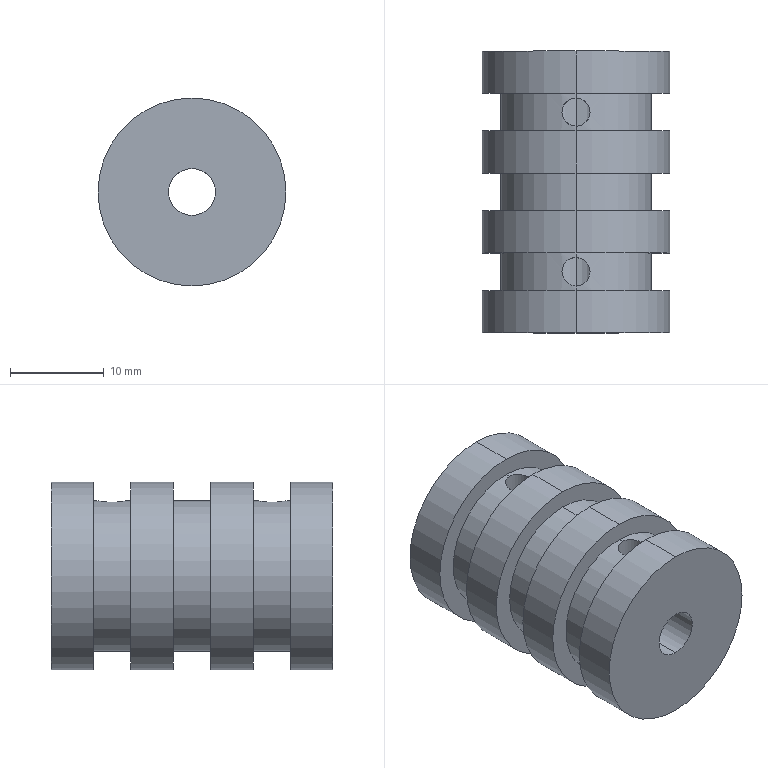Part | SolidWorks | features ICE 1, Revolution 1 | 1 solid | 31 faces | box 20 x 30 x 20 mm | volume 6534 mm3 | cylinder 22 | plane 9 | commonest cylinder face diameters 20 x8 16 x6 3 x4 5 x2 10 x2
STEP:
#1=CARTESIAN_POINT('',(0.,5.,8.));
#2=VERTEX_POINT('',#1);
#3=CARTESIAN_POINT('',(1.5,6.5,7.858));
#4=VERTEX_POINT('',#3);
#5=CARTESIAN_POINT('',(0.,5.,8.));
#6=CARTESIAN_POINT('',(0.09806,5.,8.));
#7=CARTESIAN_POINT('',(0.1977,5.01,7.998));
#8=CARTESIAN_POINT('',(0.3902,5.048,7.991));
#9=CARTESIAN_POINT('',(0.4838,5.077,7.986));
#10=CARTESIAN_POINT('',(0.7565,5.19,7.966));
#11=CARTESIAN_POINT('',(0.9215,5.3,7.948));
#12=CARTESIAN_POINT('',(1.131,5.509,7.92));
#13=CARTESIAN_POINT('',(1.193,5.585,7.911));
#14=CARTESIAN_POINT('',(1.301,5.747,7.894));
#15=CARTESIAN_POINT('',(1.348,5.835,7.886));
#16=CARTESIAN_POINT('',(1.423,6.016,7.872));
#17=CARTESIAN_POINT('',(1.452,6.11,7.867));
#18=CARTESIAN_POINT('',(1.49,6.302,7.86));
#19=CARTESIAN_POINT('',(1.5,6.402,7.858));
#20=CARTESIAN_POINT('',(1.5,6.5,7.858));
#21=B_SPLINE_CURVE_WITH_KNOTS('',3,(#5,#6,#7,#8,#9,#10,#11,#12,#13,#14,#15,#16,#17,#18,#19,#20),.UNSPECIFIED.,.F.,.F.,(4,2,2,2,2,2,2,4),(0.002351,0.002644,0.002938,0.003525,0.003819,0.004113,0.004406,0.0047),.UNSPECIFIED.);
#22=EDGE_CURVE('',#2,#4,#21,.T.);
#23=ORIENTED_EDGE('',*,*,#22,.T.);
#24=CARTESIAN_POINT('',(1.5,6.5,2.));
#25=VERTEX_POINT('',#24);
#26=CARTESIAN_POINT('',(1.5,6.5,10.001));
#27=DIRECTION('',(0.,0.,-1.));
#28=VECTOR('',#27,1000.);
#29=LINE('',#26,#28);
#30=EDGE_CURVE('',#4,#25,#29,.T.);
#31=ORIENTED_EDGE('',*,*,#30,.T.);
#32=CARTESIAN_POINT('',(0.,5.,2.5));
#33=VERTEX_POINT('',#32);
#34=CARTESIAN_POINT('',(1.5,6.5,2.));
#35=CARTESIAN_POINT('',(1.5,6.398,2.));
#36=CARTESIAN_POINT('',(1.49,6.298,2.008));
#37=CARTESIAN_POINT('',(1.45,6.103,2.037));
#38=CARTESIAN_POINT('',(1.42,6.007,2.058));
#39=CARTESIAN_POINT('',(1.306,5.737,2.134));
#40=CARTESIAN_POINT('',(1.197,5.576,2.2));
#41=CARTESIAN_POINT('',(0.994,5.373,2.295));
#42=CARTESIAN_POINT('',(0.9189,5.311,2.327));
#43=CARTESIAN_POINT('',(0.7595,5.203,2.383));
#44=CARTESIAN_POINT('',(0.6745,5.157,2.409));
#45=CARTESIAN_POINT('',(0.4928,5.08,2.453));
#46=CARTESIAN_POINT('',(0.3966,5.05,2.47));
#47=CARTESIAN_POINT('',(0.2019,5.01,2.494));
#48=CARTESIAN_POINT('',(0.1018,5.,2.5));
#49=CARTESIAN_POINT('',(0.,5.,2.5));
#50=B_SPLINE_CURVE_WITH_KNOTS('',3,(#34,#35,#36,#37,#38,#39,#40,#41,#42,#43,#44,#45,#46,#47,#48,#49),.UNSPECIFIED.,.F.,.F.,(4,2,2,2,2,2,2,4),(0.00481,0.005111,0.005411,0.006011,0.006311,0.006612,0.006912,0.007212),.UNSPECIFIED.);
#51=EDGE_CURVE('',#25,#33,#50,.T.);
#52=ORIENTED_EDGE('',*,*,#51,.T.);
#53=CARTESIAN_POINT('',(-1.5,6.5,2.));
#54=VERTEX_POINT('',#53);
#55=CARTESIAN_POINT('',(0.,5.,2.5));
#56=CARTESIAN_POINT('',(-0.1017,5.,2.5));
#57=CARTESIAN_POINT('',(-0.2015,5.01,2.494));
#58=CARTESIAN_POINT('',(-0.3974,5.05,2.47));
#59=CARTESIAN_POINT('',(-0.494,5.08,2.452));
#60=CARTESIAN_POINT('',(-0.7657,5.195,2.387));
#61=CARTESIAN_POINT('',(-0.9285,5.306,2.326));
#62=CARTESIAN_POINT('',(-1.131,5.51,2.231));
#63=CARTESIAN_POINT('',(-1.192,5.585,2.198));
#64=CARTESIAN_POINT('',(-1.299,5.744,2.137));
#65=CARTESIAN_POINT('',(-1.345,5.828,2.108));
#66=CARTESIAN_POINT('',(-1.421,6.008,2.058));
#67=CARTESIAN_POINT('',(-1.45,6.104,2.037));
#68=CARTESIAN_POINT('',(-1.49,6.298,2.008));
#69=CARTESIAN_POINT('',(-1.5,6.398,2.));
#70=CARTESIAN_POINT('',(-1.5,6.5,2.));
#71=B_SPLINE_CURVE_WITH_KNOTS('',3,(#55,#56,#57,#58,#59,#60,#61,#62,#63,#64,#65,#66,#67,#68,#69,#70),.UNSPECIFIED.,.F.,.F.,(4,2,2,2,2,2,2,4),(0.007212,0.007512,0.007812,0.008412,0.008712,0.009012,0.009312,0.009612),.UNSPECIFIED.);
#72=EDGE_CURVE('',#33,#54,#71,.T.);
#73=ORIENTED_EDGE('',*,*,#72,.T.);
#74=CARTESIAN_POINT('',(-1.5,6.5,7.858));
#75=VERTEX_POINT('',#74);
#76=CARTESIAN_POINT('',(-1.5,6.5,10.001));
#77=DIRECTION('',(0.,0.,-1.));
#78=VECTOR('',#77,1000.);
#79=LINE('',#76,#78);
#80=EDGE_CURVE('',#75,#54,#79,.T.);
#81=ORIENTED_EDGE('',*,*,#80,.F.);
#82=CARTESIAN_POINT('',(-1.5,6.5,7.858));
#83=CARTESIAN_POINT('',(-1.5,6.401,7.858));
#84=CARTESIAN_POINT('',(-1.49,6.303,7.86));
#85=CARTESIAN_POINT('',(-1.452,6.111,7.867));
#86=CARTESIAN_POINT('',(-1.423,6.015,7.873));
#87=CARTESIAN_POINT('',(-1.348,5.834,7.886));
#88=CARTESIAN_POINT('',(-1.301,5.748,7.894));
#89=CARTESIAN_POINT('',(-1.193,5.585,7.911));
#90=CARTESIAN_POINT('',(-1.129,5.508,7.92));
#91=CARTESIAN_POINT('',(-0.9221,5.301,7.948));
#92=CARTESIAN_POINT('',(-0.755,5.189,7.966));
#93=CARTESIAN_POINT('',(-0.394,5.04,7.992));
#94=CARTESIAN_POINT('',(-0.1962,5.,8.));
#95=CARTESIAN_POINT('',(0.,5.,8.));
#96=B_SPLINE_CURVE_WITH_KNOTS('',3,(#82,#83,#84,#85,#86,#87,#88,#89,#90,#91,#92,#93,#94,#95),.UNSPECIFIED.,.F.,.F.,(4,2,2,2,2,2,4),(0.,0.0002938,0.0005877,0.0008815,0.001175,0.001763,0.002351),.UNSPECIFIED.);
#97=EDGE_CURVE('',#75,#2,#96,.T.);
#98=ORIENTED_EDGE('',*,*,#97,.T.);
#99=EDGE_LOOP('',(#23,#31,#52,#73,#81,#98));
#100=FACE_OUTER_BOUND('',#99,.T.);
#101=CARTESIAN_POINT('',(0.,6.5,10.001));
#102=DIRECTION('',(0.,0.,-1.));
#103=DIRECTION('',(-1.,0.,0.));
#104=AXIS2_PLACEMENT_3D('',#101,#102,#103);
#105=CYLINDRICAL_SURFACE('',#104,1.5);
#106=ADVANCED_FACE('',(#100),#105,.F.);
#107=CARTESIAN_POINT('',(0.,22.,8.));
#108=VERTEX_POINT('',#107);
#109=CARTESIAN_POINT('',(1.5,23.5,7.858));
#110=VERTEX_POINT('',#109);
#111=CARTESIAN_POINT('',(0.,22.,8.));
#112=CARTESIAN_POINT('',(0.09806,22.,8.));
#113=CARTESIAN_POINT('',(0.1977,22.01,7.998));
#114=CARTESIAN_POINT('',(0.3902,22.048,7.991));
#115=CARTESIAN_POINT('',(0.4838,22.077,7.986));
#116=CARTESIAN_POINT('',(0.7565,22.19,7.966));
#117=CARTESIAN_POINT('',(0.9215,22.3,7.948));
#118=CARTESIAN_POINT('',(1.131,22.509,7.92));
#119=CARTESIAN_POINT('',(1.193,22.585,7.911));
#120=CARTESIAN_POINT('',(1.301,22.747,7.894));
#121=CARTESIAN_POINT('',(1.348,22.835,7.886));
#122=CARTESIAN_POINT('',(1.423,23.016,7.872));
#123=CARTESIAN_POINT('',(1.452,23.11,7.867));
#124=CARTESIAN_POINT('',(1.49,23.302,7.86));
#125=CARTESIAN_POINT('',(1.5,23.402,7.858));
#126=CARTESIAN_POINT('',(1.5,23.5,7.858));
#127=B_SPLINE_CURVE_WITH_KNOTS('',3,(#111,#112,#113,#114,#115,#116,#117,#118,#119,#120,#121,#122,#123,#124,#125,#126),.UNSPECIFIED.,.F.,.F.,(4,2,2,2,2,2,2,4),(0.002351,0.002644,0.002938,0.003525,0.003819,0.004113,0.004406,0.0047),.UNSPECIFIED.);
#128=EDGE_CURVE('',#108,#110,#127,.T.);
#129=ORIENTED_EDGE('',*,*,#128,.T.);
#130=CARTESIAN_POINT('',(1.5,23.5,4.77));
#131=VERTEX_POINT('',#130);
#132=CARTESIAN_POINT('',(1.5,23.5,10.001));
#133=DIRECTION('',(0.,0.,-1.));
#134=VECTOR('',#133,1000.);
#135=LINE('',#132,#134);
#136=EDGE_CURVE('',#110,#131,#135,.T.);
#137=ORIENTED_EDGE('',*,*,#136,.T.);
#138=CARTESIAN_POINT('',(0.,22.,5.));
#139=VERTEX_POINT('',#138);
#140=CARTESIAN_POINT('',(1.5,23.5,4.77));
#141=CARTESIAN_POINT('',(1.5,23.304,4.77));
#142=CARTESIAN_POINT('',(1.46,23.105,4.783));
#143=CARTESIAN_POINT('',(1.348,22.834,4.815));
#144=CARTESIAN_POINT('',(1.301,22.746,4.828));
#145=CARTESIAN_POINT('',(1.192,22.584,4.856));
#146=CARTESIAN_POINT('',(1.13,22.509,4.871));
#147=CARTESIAN_POINT('',(0.9225,22.301,4.916));
#148=CARTESIAN_POINT('',(0.759,22.191,4.945));
#149=CARTESIAN_POINT('',(0.4847,22.077,4.977));
#150=CARTESIAN_POINT('',(0.3908,22.048,4.986));
#151=CARTESIAN_POINT('',(0.1985,22.01,4.997));
#152=CARTESIAN_POINT('',(0.09886,22.,5.));
#153=CARTESIAN_POINT('',(0.,22.,5.));
#154=B_SPLINE_CURVE_WITH_KNOTS('',3,(#140,#141,#142,#143,#144,#145,#146,#147,#148,#149,#150,#151,#152,#153),.UNSPECIFIED.,.F.,.F.,(4,2,2,2,2,2,4),(0.004717,0.005306,0.005601,0.005896,0.006485,0.00678,0.007075),.UNSPECIFIED.);
#155=EDGE_CURVE('',#131,#139,#154,.T.);
#156=ORIENTED_EDGE('',*,*,#155,.T.);
#157=CARTESIAN_POINT('',(-1.5,23.5,4.77));
#158=VERTEX_POINT('',#157);
#159=CARTESIAN_POINT('',(0.,22.,5.));
#160=CARTESIAN_POINT('',(-0.09885,22.,5.));
#161=CARTESIAN_POINT('',(-0.1966,22.01,4.997));
#162=CARTESIAN_POINT('',(-0.3899,22.048,4.986));
#163=CARTESIAN_POINT('',(-0.4856,22.077,4.977));
#164=CARTESIAN_POINT('',(-0.7566,22.19,4.946));
#165=CARTESIAN_POINT('',(-0.9229,22.302,4.916));
#166=CARTESIAN_POINT('',(-1.129,22.508,4.871));
#167=CARTESIAN_POINT('',(-1.192,22.584,4.856));
#168=CARTESIAN_POINT('',(-1.301,22.747,4.828));
#169=CARTESIAN_POINT('',(-1.347,22.833,4.815));
#170=CARTESIAN_POINT('',(-1.422,23.014,4.794));
#171=CARTESIAN_POINT('',(-1.452,23.109,4.785));
#172=CARTESIAN_POINT('',(-1.49,23.302,4.773));
#173=CARTESIAN_POINT('',(-1.5,23.4,4.77));
#174=CARTESIAN_POINT('',(-1.5,23.5,4.77));
#175=B_SPLINE_CURVE_WITH_KNOTS('',3,(#159,#160,#161,#162,#163,#164,#165,#166,#167,#168,#169,#170,#171,#172,#173,#174),.UNSPECIFIED.,.F.,.F.,(4,2,2,2,2,2,2,4),(0.007075,0.00737,0.007664,0.008254,0.008548,0.008843,0.009138,0.009433),.UNSPECIFIED.);
#176=EDGE_CURVE('',#139,#158,#175,.T.);
#177=ORIENTED_EDGE('',*,*,#176,.T.);
#178=CARTESIAN_POINT('',(-1.5,23.5,7.858));
#179=VERTEX_POINT('',#178);
#180=CARTESIAN_POINT('',(-1.5,23.5,10.001));
#181=DIRECTION('',(0.,0.,-1.));
#182=VECTOR('',#181,1000.);
#183=LINE('',#180,#182);
#184=EDGE_CURVE('',#179,#158,#183,.T.);
#185=ORIENTED_EDGE('',*,*,#184,.F.);
#186=CARTESIAN_POINT('',(-1.5,23.5,7.858));
#187=CARTESIAN_POINT('',(-1.5,23.401,7.858));
#188=CARTESIAN_POINT('',(-1.49,23.303,7.86));
#189=CARTESIAN_POINT('',(-1.452,23.111,7.867));
#190=CARTESIAN_POINT('',(-1.423,23.015,7.873));
#191=CARTESIAN_POINT('',(-1.348,22.834,7.886));
#192=CARTESIAN_POINT('',(-1.301,22.748,7.894));
#193=CARTESIAN_POINT('',(-1.193,22.585,7.911));
#194=CARTESIAN_POINT('',(-1.129,22.508,7.92));
#195=CARTESIAN_POINT('',(-0.9221,22.301,7.948));
#196=CARTESIAN_POINT('',(-0.755,22.189,7.966));
#197=CARTESIAN_POINT('',(-0.394,22.04,7.992));
#198=CARTESIAN_POINT('',(-0.1962,22.,8.));
#199=CARTESIAN_POINT('',(0.,22.,8.));
#200=B_SPLINE_CURVE_WITH_KNOTS('',3,(#186,#187,#188,#189,#190,#191,#192,#193,#194,#195,#196,#197,#198,#199),.UNSPECIFIED.,.F.,.F.,(4,2,2,2,2,2,4),(0.,0.0002938,0.0005877,0.0008815,0.001175,0.001763,0.002351),.UNSPECIFIED.);
#201=EDGE_CURVE('',#179,#108,#200,.T.);
#202=ORIENTED_EDGE('',*,*,#201,.T.);
#203=EDGE_LOOP('',(#129,#137,#156,#177,#185,#202));
#204=FACE_OUTER_BOUND('',#203,.T.);
#205=CARTESIAN_POINT('',(0.,23.5,10.001));
#206=DIRECTION('',(0.,0.,-1.));
#207=DIRECTION('',(-1.,0.,0.));
#208=AXIS2_PLACEMENT_3D('',#205,#206,#207);
#209=CYLINDRICAL_SURFACE('',#208,1.5);
#210=ADVANCED_FACE('',(#204),#209,.F.);
#211=CARTESIAN_POINT('',(0.,30.,-10.));
#212=VERTEX_POINT('',#211);
#213=CARTESIAN_POINT('',(0.,30.,10.));
#214=VERTEX_POINT('',#213);
#215=CARTESIAN_POINT('',(0.,30.,0.));
#216=DIRECTION('',(0.,-1.,0.));
#217=DIRECTION('',(0.,0.,-1.));
#218=AXIS2_PLACEMENT_3D('',#215,#216,#217);
#219=CIRCLE('',#218,10.);
#220=EDGE_CURVE('',#212,#214,#219,.T.);
#221=ORIENTED_EDGE('',*,*,#220,.T.);
#222=CARTESIAN_POINT('',(0.,25.5,10.));
#223=VERTEX_POINT('',#222);
#224=CARTESIAN_POINT('',(0.,0.,10.));
#225=DIRECTION('',(0.,-1.,0.));
#226=VECTOR('',#225,1000.);
#227=LINE('',#224,#226);
#228=EDGE_CURVE('',#214,#223,#227,.T.);
#229=ORIENTED_EDGE('',*,*,#228,.T.);
#230=CARTESIAN_POINT('',(0.,25.5,-10.));
#231=VERTEX_POINT('',#230);
#232=CARTESIAN_POINT('',(0.,25.5,0.));
#233=DIRECTION('',(0.,-1.,0.));
#234=DIRECTION('',(0.,0.,-1.));
#235=AXIS2_PLACEMENT_3D('',#232,#233,#234);
#236=CIRCLE('',#235,10.);
#237=EDGE_CURVE('',#231,#223,#236,.T.);
#238=ORIENTED_EDGE('',*,*,#237,.F.);
#239=CARTESIAN_POINT('',(0.,0.,-10.));
#240=DIRECTION('',(0.,-1.,0.));
#241=VECTOR('',#240,1000.);
#242=LINE('',#239,#241);
#243=EDGE_CURVE('',#212,#231,#242,.T.);
#244=ORIENTED_EDGE('',*,*,#243,.F.);
#245=EDGE_LOOP('',(#221,#229,#238,#244));
#246=FACE_OUTER_BOUND('',#245,.T.);
#247=CARTESIAN_POINT('',(0.,0.,0.));
#248=DIRECTION('',(0.,-1.,0.));
#249=DIRECTION('',(0.,0.,-1.));
#250=AXIS2_PLACEMENT_3D('',#247,#248,#249);
#251=CYLINDRICAL_SURFACE('',#250,10.);
#252=ADVANCED_FACE('',(#246),#251,.T.);
#253=CARTESIAN_POINT('',(0.,21.5,-10.));
#254=VERTEX_POINT('',#253);
#255=CARTESIAN_POINT('',(0.,21.5,10.));
#256=VERTEX_POINT('',#255);
#257=CARTESIAN_POINT('',(0.,21.5,0.));
#258=DIRECTION('',(0.,-1.,0.));
#259=DIRECTION('',(0.,0.,-1.));
#260=AXIS2_PLACEMENT_3D('',#257,#258,#259);
#261=CIRCLE('',#260,10.);
#262=EDGE_CURVE('',#254,#256,#261,.T.);
#263=ORIENTED_EDGE('',*,*,#262,.T.);
#264=CARTESIAN_POINT('',(0.,17.,10.));
#265=VERTEX_POINT('',#264);
#266=CARTESIAN_POINT('',(0.,0.,10.));
#267=DIRECTION('',(0.,-1.,0.));
#268=VECTOR('',#267,1000.);
#269=LINE('',#266,#268);
#270=EDGE_CURVE('',#256,#265,#269,.T.);
#271=ORIENTED_EDGE('',*,*,#270,.T.);
#272=CARTESIAN_POINT('',(0.,17.,-10.));
#273=VERTEX_POINT('',#272);
#274=CARTESIAN_POINT('',(0.,17.,0.));
#275=DIRECTION('',(0.,-1.,0.));
#276=DIRECTION('',(0.,0.,-1.));
#277=AXIS2_PLACEMENT_3D('',#274,#275,#276);
#278=CIRCLE('',#277,10.);
#279=EDGE_CURVE('',#273,#265,#278,.T.);
#280=ORIENTED_EDGE('',*,*,#279,.F.);
#281=CARTESIAN_POINT('',(0.,0.,-10.));
#282=DIRECTION('',(0.,-1.,0.));
#283=VECTOR('',#282,1000.);
#284=LINE('',#281,#283);
#285=EDGE_CURVE('',#254,#273,#284,.T.);
#286=ORIENTED_EDGE('',*,*,#285,.F.);
#287=EDGE_LOOP('',(#263,#271,#280,#286));
#288=FACE_OUTER_BOUND('',#287,.T.);
#289=CARTESIAN_POINT('',(0.,0.,0.));
#290=DIRECTION('',(0.,-1.,0.));
#291=DIRECTION('',(0.,0.,-1.));
#292=AXIS2_PLACEMENT_3D('',#289,#290,#291);
#293=CYLINDRICAL_SURFACE('',#292,10.);
#294=ADVANCED_FACE('',(#288),#293,.T.);
#295=CARTESIAN_POINT('',(0.,17.,-8.));
#296=VERTEX_POINT('',#295);
#297=CARTESIAN_POINT('',(0.,17.,8.));
#298=VERTEX_POINT('',#297);
#299=CARTESIAN_POINT('',(0.,17.,0.));
#300=DIRECTION('',(0.,-1.,0.));
#301=DIRECTION('',(0.,0.,-1.));
#302=AXIS2_PLACEMENT_3D('',#299,#300,#301);
#303=CIRCLE('',#302,8.);
#304=EDGE_CURVE('',#296,#298,#303,.T.);
#305=ORIENTED_EDGE('',*,*,#304,.T.);
#306=CARTESIAN_POINT('',(0.,13.,8.));
#307=VERTEX_POINT('',#306);
#308=CARTESIAN_POINT('',(0.,0.,8.));
#309=DIRECTION('',(0.,-1.,0.));
#310=VECTOR('',#309,1000.);
#311=LINE('',#308,#310);
#312=EDGE_CURVE('',#298,#307,#311,.T.);
#313=ORIENTED_EDGE('',*,*,#312,.T.);
#314=CARTESIAN_POINT('',(0.,13.,-8.));
#315=VERTEX_POINT('',#314);
#316=CARTESIAN_POINT('',(0.,13.,0.));
#317=DIRECTION('',(0.,-1.,0.));
#318=DIRECTION('',(0.,0.,-1.));
#319=AXIS2_PLACEMENT_3D('',#316,#317,#318);
#320=CIRCLE('',#319,8.);
#321=EDGE_CURVE('',#315,#307,#320,.T.);
#322=ORIENTED_EDGE('',*,*,#321,.F.);
#323=CARTESIAN_POINT('',(0.,0.,-8.));
#324=DIRECTION('',(0.,-1.,0.));
#325=VECTOR('',#324,1000.);
#326=LINE('',#323,#325);
#327=EDGE_CURVE('',#296,#315,#326,.T.);
#328=ORIENTED_EDGE('',*,*,#327,.F.);
#329=EDGE_LOOP('',(#305,#313,#322,#328));
#330=FACE_OUTER_BOUND('',#329,.T.);
#331=CARTESIAN_POINT('',(0.,0.,0.));
#332=DIRECTION('',(0.,-1.,0.));
#333=DIRECTION('',(0.,0.,-1.));
#334=AXIS2_PLACEMENT_3D('',#331,#332,#333);
#335=CYLINDRICAL_SURFACE('',#334,8.);
#336=ADVANCED_FACE('',(#330),#335,.T.);
#337=CARTESIAN_POINT('',(0.,13.,-10.));
#338=VERTEX_POINT('',#337);
#339=CARTESIAN_POINT('',(0.,13.,10.));
#340=VERTEX_POINT('',#339);
#341=CARTESIAN_POINT('',(0.,13.,0.));
#342=DIRECTION('',(0.,-1.,0.));
#343=DIRECTION('',(0.,0.,-1.));
#344=AXIS2_PLACEMENT_3D('',#341,#342,#343);
#345=CIRCLE('',#344,10.);
#346=EDGE_CURVE('',#338,#340,#345,.T.);
#347=ORIENTED_EDGE('',*,*,#346,.T.);
#348=CARTESIAN_POINT('',(0.,8.5,10.));
#349=VERTEX_POINT('',#348);
#350=CARTESIAN_POINT('',(0.,0.,10.));
#351=DIRECTION('',(0.,-1.,0.));
#352=VECTOR('',#351,1000.);
#353=LINE('',#350,#352);
#354=EDGE_CURVE('',#340,#349,#353,.T.);
#355=ORIENTED_EDGE('',*,*,#354,.T.);
#356=CARTESIAN_POINT('',(0.,8.5,-10.));
#357=VERTEX_POINT('',#356);
#358=CARTESIAN_POINT('',(0.,8.5,0.));
#359=DIRECTION('',(0.,-1.,0.));
#360=DIRECTION('',(0.,0.,-1.));
#361=AXIS2_PLACEMENT_3D('',#358,#359,#360);
#362=CIRCLE('',#361,10.);
#363=EDGE_CURVE('',#357,#349,#362,.T.);
#364=ORIENTED_EDGE('',*,*,#363,.F.);
#365=CARTESIAN_POINT('',(0.,0.,-10.));
#366=DIRECTION('',(0.,-1.,0.));
#367=VECTOR('',#366,1000.);
#368=LINE('',#365,#367);
#369=EDGE_CURVE('',#338,#357,#368,.T.);
#370=ORIENTED_EDGE('',*,*,#369,.F.);
#371=EDGE_LOOP('',(#347,#355,#364,#370));
#372=FACE_OUTER_BOUND('',#371,.T.);
#373=CARTESIAN_POINT('',(0.,0.,0.));
#374=DIRECTION('',(0.,-1.,0.));
#375=DIRECTION('',(0.,0.,-1.));
#376=AXIS2_PLACEMENT_3D('',#373,#374,#375);
#377=CYLINDRICAL_SURFACE('',#376,10.);
#378=ADVANCED_FACE('',(#372),#377,.T.);
#379=CARTESIAN_POINT('',(0.,4.5,-10.));
#380=VERTEX_POINT('',#379);
#381=CARTESIAN_POINT('',(0.,4.5,10.));
#382=VERTEX_POINT('',#381);
#383=CARTESIAN_POINT('',(0.,4.5,0.));
#384=DIRECTION('',(0.,-1.,0.));
#385=DIRECTION('',(0.,0.,-1.));
#386=AXIS2_PLACEMENT_3D('',#383,#384,#385);
#387=CIRCLE('',#386,10.);
#388=EDGE_CURVE('',#380,#382,#387,.T.);
#389=ORIENTED_EDGE('',*,*,#388,.T.);
#390=CARTESIAN_POINT('',(0.,0.,10.));
#391=VERTEX_POINT('',#390);
#392=CARTESIAN_POINT('',(0.,0.,10.));
#393=DIRECTION('',(0.,-1.,0.));
#394=VECTOR('',#393,1000.);
#395=LINE('',#392,#394);
#396=EDGE_CURVE('',#382,#391,#395,.T.);
#397=ORIENTED_EDGE('',*,*,#396,.T.);
#398=CARTESIAN_POINT('',(0.,0.,-10.));
#399=VERTEX_POINT('',#398);
#400=CARTESIAN_POINT('',(0.,0.,0.));
#401=DIRECTION('',(0.,-1.,0.));
#402=DIRECTION('',(0.,0.,-1.));
#403=AXIS2_PLACEMENT_3D('',#400,#401,#402);
#404=CIRCLE('',#403,10.);
#405=EDGE_CURVE('',#399,#391,#404,.T.);
#406=ORIENTED_EDGE('',*,*,#405,.F.);
#407=CARTESIAN_POINT('',(0.,0.,-10.));
#408=DIRECTION('',(0.,-1.,0.));
#409=VECTOR('',#408,1000.);
#410=LINE('',#407,#409);
#411=EDGE_CURVE('',#380,#399,#410,.T.);
#412=ORIENTED_EDGE('',*,*,#411,.F.);
#413=EDGE_LOOP('',(#389,#397,#406,#412));
#414=FACE_OUTER_BOUND('',#413,.T.);
#415=CARTESIAN_POINT('',(0.,0.,0.));
#416=DIRECTION('',(0.,-1.,0.));
#417=DIRECTION('',(0.,0.,-1.));
#418=AXIS2_PLACEMENT_3D('',#415,#416,#417);
#419=CYLINDRICAL_SURFACE('',#418,10.);
#420=ADVANCED_FACE('',(#414),#419,.T.);
#421=CARTESIAN_POINT('',(0.,30.,5.));
#422=VERTEX_POINT('',#421);
#423=CARTESIAN_POINT('',(0.,30.,-5.));
#424=VERTEX_POINT('',#423);
#425=CARTESIAN_POINT('',(0.,30.,0.));
#426=DIRECTION('',(0.,-1.,0.));
#427=DIRECTION('',(0.,0.,-1.));
#428=AXIS2_PLACEMENT_3D('',#425,#426,#427);
#429=CIRCLE('',#428,5.);
#430=EDGE_CURVE('',#422,#424,#429,.T.);
#431=ORIENTED_EDGE('',*,*,#430,.F.);
#432=CARTESIAN_POINT('',(0.,25.,5.));
#433=VERTEX_POINT('',#432);
#434=CARTESIAN_POINT('',(0.,0.,5.));
#435=DIRECTION('',(0.,-1.,0.));
#436=VECTOR('',#435,1000.);
#437=LINE('',#434,#436);
#438=EDGE_CURVE('',#422,#433,#437,.T.);
#439=ORIENTED_EDGE('',*,*,#438,.T.);
#440=CARTESIAN_POINT('',(-1.5,23.5,4.77));
#441=CARTESIAN_POINT('',(-1.5,23.6,4.77));
#442=CARTESIAN_POINT('',(-1.49,23.698,4.773));
#443=CARTESIAN_POINT('',(-1.452,23.89,4.785));
#444=CARTESIAN_POINT('',(-1.423,23.986,4.794));
#445=CARTESIAN_POINT('',(-1.347,24.167,4.815));
#446=CARTESIAN_POINT('',(-1.301,24.253,4.828));
#447=CARTESIAN_POINT('',(-1.192,24.416,4.856));
#448=CARTESIAN_POINT('',(-1.129,24.492,4.871));
#449=CARTESIAN_POINT('',(-0.9226,24.699,4.916));
#450=CARTESIAN_POINT('',(-0.7561,24.81,4.946));
#451=CARTESIAN_POINT('',(-0.3953,24.96,4.988));
#452=CARTESIAN_POINT('',(-0.197,25.,5.));
#453=CARTESIAN_POINT('',(0.,25.,5.));
#454=B_SPLINE_CURVE_WITH_KNOTS('',3,(#440,#441,#442,#443,#444,#445,#446,#447,#448,#449,#450,#451,#452,#453),.UNSPECIFIED.,.F.,.F.,(4,2,2,2,2,2,4),(0.,0.0002949,0.0005898,0.0008847,0.00118,0.001769,0.002359),.UNSPECIFIED.);
#455=EDGE_CURVE('',#158,#433,#454,.T.);
#456=ORIENTED_EDGE('',*,*,#455,.F.);
#457=ORIENTED_EDGE('',*,*,#176,.F.);
#458=CARTESIAN_POINT('',(0.,15.,5.));
#459=VERTEX_POINT('',#458);
#460=CARTESIAN_POINT('',(0.,0.,5.));
#461=DIRECTION('',(0.,-1.,0.));
#462=VECTOR('',#461,1000.);
#463=LINE('',#460,#462);
#464=EDGE_CURVE('',#139,#459,#463,.T.);
#465=ORIENTED_EDGE('',*,*,#464,.T.);
#466=CARTESIAN_POINT('',(0.,15.,-5.));
#467=VERTEX_POINT('',#466);
#468=CARTESIAN_POINT('',(0.,15.,0.));
#469=DIRECTION('',(0.,-1.,0.));
#470=DIRECTION('',(0.,0.,-1.));
#471=AXIS2_PLACEMENT_3D('',#468,#469,#470);
#472=CIRCLE('',#471,5.);
#473=EDGE_CURVE('',#459,#467,#472,.T.);
#474=ORIENTED_EDGE('',*,*,#473,.T.);
#475=CARTESIAN_POINT('',(0.,0.,-5.));
#476=DIRECTION('',(0.,-1.,0.));
#477=VECTOR('',#476,1000.);
#478=LINE('',#475,#477);
#479=EDGE_CURVE('',#424,#467,#478,.T.);
#480=ORIENTED_EDGE('',*,*,#479,.F.);
#481=EDGE_LOOP('',(#431,#439,#456,#457,#465,#474,#480));
#482=FACE_OUTER_BOUND('',#481,.T.);
#483=CARTESIAN_POINT('',(0.,0.,0.));
#484=DIRECTION('',(0.,-1.,0.));
#485=DIRECTION('',(0.,0.,-1.));
#486=AXIS2_PLACEMENT_3D('',#483,#484,#485);
#487=CYLINDRICAL_SURFACE('',#486,5.);
#488=ADVANCED_FACE('',(#482),#487,.F.);
#489=CARTESIAN_POINT('',(0.,25.5,-8.));
#490=VERTEX_POINT('',#489);
#491=CARTESIAN_POINT('',(0.,25.5,8.));
#492=VERTEX_POINT('',#491);
#493=CARTESIAN_POINT('',(0.,25.5,0.));
#494=DIRECTION('',(0.,-1.,0.));
#495=DIRECTION('',(0.,0.,-1.));
#496=AXIS2_PLACEMENT_3D('',#493,#494,#495);
#497=CIRCLE('',#496,8.);
#498=EDGE_CURVE('',#490,#492,#497,.T.);
#499=ORIENTED_EDGE('',*,*,#498,.T.);
#500=CARTESIAN_POINT('',(0.,25.,8.));
#501=VERTEX_POINT('',#500);
#502=CARTESIAN_POINT('',(0.,0.,8.));
#503=DIRECTION('',(0.,-1.,0.));
#504=VECTOR('',#503,1000.);
#505=LINE('',#502,#504);
#506=EDGE_CURVE('',#492,#501,#505,.T.);
#507=ORIENTED_EDGE('',*,*,#506,.T.);
#508=CARTESIAN_POINT('',(1.5,23.5,7.858));
#509=CARTESIAN_POINT('',(1.5,23.696,7.858));
#510=CARTESIAN_POINT('',(1.461,23.894,7.866));
#511=CARTESIAN_POINT('',(1.311,24.255,7.892));
#512=CARTESIAN_POINT('',(1.199,24.422,7.911));
#513=CARTESIAN_POINT('',(0.9919,24.629,7.939));
#514=CARTESIAN_POINT('',(0.9149,24.693,7.948));
#515=CARTESIAN_POINT('',(0.7523,24.801,7.965));
#516=CARTESIAN_POINT('',(0.6663,24.848,7.973));
#517=CARTESIAN_POINT('',(0.3933,24.961,7.992));
#518=CARTESIAN_POINT('',(0.1982,25.,8.));
#519=CARTESIAN_POINT('',(0.,25.,8.));
#520=B_SPLINE_CURVE_WITH_KNOTS('',3,(#508,#509,#510,#511,#512,#513,#514,#515,#516,#517,#518,#519),.UNSPECIFIED.,.F.,.F.,(4,2,2,2,2,4),(0.0047,0.005288,0.005875,0.006169,0.006463,0.00705),.UNSPECIFIED.);
#521=EDGE_CURVE('',#110,#501,#520,.T.);
#522=ORIENTED_EDGE('',*,*,#521,.F.);
#523=ORIENTED_EDGE('',*,*,#128,.F.);
#524=CARTESIAN_POINT('',(0.,21.5,8.));
#525=VERTEX_POINT('',#524);
#526=CARTESIAN_POINT('',(0.,0.,8.));
#527=DIRECTION('',(0.,-1.,0.));
#528=VECTOR('',#527,1000.);
#529=LINE('',#526,#528);
#530=EDGE_CURVE('',#108,#525,#529,.T.);
#531=ORIENTED_EDGE('',*,*,#530,.T.);
#532=CARTESIAN_POINT('',(0.,21.5,-8.));
#533=VERTEX_POINT('',#532);
#534=CARTESIAN_POINT('',(0.,21.5,0.));
#535=DIRECTION('',(0.,-1.,0.));
#536=DIRECTION('',(0.,0.,-1.));
#537=AXIS2_PLACEMENT_3D('',#534,#535,#536);
#538=CIRCLE('',#537,8.);
#539=EDGE_CURVE('',#533,#525,#538,.T.);
#540=ORIENTED_EDGE('',*,*,#539,.F.);
#541=CARTESIAN_POINT('',(0.,0.,-8.));
#542=DIRECTION('',(0.,-1.,0.));
#543=VECTOR('',#542,1000.);
#544=LINE('',#541,#543);
#545=EDGE_CURVE('',#490,#533,#544,.T.);
#546=ORIENTED_EDGE('',*,*,#545,.F.);
#547=EDGE_LOOP('',(#499,#507,#522,#523,#531,#540,#546));
#548=FACE_OUTER_BOUND('',#547,.T.);
#549=CARTESIAN_POINT('',(0.,0.,0.));
#550=DIRECTION('',(0.,-1.,0.));
#551=DIRECTION('',(0.,0.,-1.));
#552=AXIS2_PLACEMENT_3D('',#549,#550,#551);
#553=CYLINDRICAL_SURFACE('',#552,8.);
#554=ADVANCED_FACE('',(#548),#553,.T.);
#555=CARTESIAN_POINT('',(0.,15.,2.5));
#556=VERTEX_POINT('',#555);
#557=CARTESIAN_POINT('',(0.,15.,-2.5));
#558=VERTEX_POINT('',#557);
#559=CARTESIAN_POINT('',(0.,15.,0.));
#560=DIRECTION('',(0.,-1.,0.));
#561=DIRECTION('',(0.,0.,-1.));
#562=AXIS2_PLACEMENT_3D('',#559,#560,#561);
#563=CIRCLE('',#562,2.5);
#564=EDGE_CURVE('',#556,#558,#563,.T.);
#565=ORIENTED_EDGE('',*,*,#564,.F.);
#566=CARTESIAN_POINT('',(0.,8.,2.5));
#567=VERTEX_POINT('',#566);
#568=CARTESIAN_POINT('',(0.,0.,2.5));
#569=DIRECTION('',(0.,-1.,0.));
#570=VECTOR('',#569,1000.);
#571=LINE('',#568,#570);
#572=EDGE_CURVE('',#556,#567,#571,.T.);
#573=ORIENTED_EDGE('',*,*,#572,.T.);
#574=CARTESIAN_POINT('',(-1.5,6.5,2.));
#575=CARTESIAN_POINT('',(-1.5,6.602,2.));
#576=CARTESIAN_POINT('',(-1.49,6.702,2.008));
#577=CARTESIAN_POINT('',(-1.45,6.897,2.037));
#578=CARTESIAN_POINT('',(-1.42,6.993,2.058));
#579=CARTESIAN_POINT('',(-1.306,7.263,2.133));
#580=CARTESIAN_POINT('',(-1.197,7.424,2.2));
#581=CARTESIAN_POINT('',(-0.9943,7.627,2.295));
#582=CARTESIAN_POINT('',(-0.9191,7.689,2.326));
#583=CARTESIAN_POINT('',(-0.7589,7.797,2.384));
#584=CARTESIAN_POINT('',(-0.6739,7.844,2.409));
#585=CARTESIAN_POINT('',(-0.4932,7.92,2.453));
#586=CARTESIAN_POINT('',(-0.3963,7.95,2.47));
#587=CARTESIAN_POINT('',(-0.2008,7.99,2.494));
#588=CARTESIAN_POINT('',(-0.1013,8.,2.5));
#589=CARTESIAN_POINT('',(0.,8.,2.5));
#590=B_SPLINE_CURVE_WITH_KNOTS('',3,(#574,#575,#576,#577,#578,#579,#580,#581,#582,#583,#584,#585,#586,#587,#588,#589),.UNSPECIFIED.,.F.,.F.,(4,2,2,2,2,2,2,4),(0.,0.000301,0.000602,0.001204,0.001505,0.001806,0.002107,0.002408),.UNSPECIFIED.);
#591=EDGE_CURVE('',#54,#567,#590,.T.);
#592=ORIENTED_EDGE('',*,*,#591,.F.);
#593=ORIENTED_EDGE('',*,*,#72,.F.);
#594=CARTESIAN_POINT('',(0.,0.,2.5));
#595=VERTEX_POINT('',#594);
#596=CARTESIAN_POINT('',(0.,0.,2.5));
#597=DIRECTION('',(0.,-1.,0.));
#598=VECTOR('',#597,1000.);
#599=LINE('',#596,#598);
#600=EDGE_CURVE('',#33,#595,#599,.T.);
#601=ORIENTED_EDGE('',*,*,#600,.T.);
#602=CARTESIAN_POINT('',(0.,0.,-2.5));
#603=VERTEX_POINT('',#602);
#604=CARTESIAN_POINT('',(0.,0.,0.));
#605=DIRECTION('',(0.,-1.,0.));
#606=DIRECTION('',(0.,0.,-1.));
#607=AXIS2_PLACEMENT_3D('',#604,#605,#606);
#608=CIRCLE('',#607,2.5);
#609=EDGE_CURVE('',#595,#603,#608,.T.);
#610=ORIENTED_EDGE('',*,*,#609,.T.);
#611=CARTESIAN_POINT('',(0.,0.,-2.5));
#612=DIRECTION('',(0.,-1.,0.));
#613=VECTOR('',#612,1000.);
#614=LINE('',#611,#613);
#615=EDGE_CURVE('',#558,#603,#614,.T.);
#616=ORIENTED_EDGE('',*,*,#615,.F.);
#617=EDGE_LOOP('',(#565,#573,#592,#593,#601,#610,#616));
#618=FACE_OUTER_BOUND('',#617,.T.);
#619=CARTESIAN_POINT('',(0.,0.,0.));
#620=DIRECTION('',(0.,-1.,0.));
#621=DIRECTION('',(0.,0.,-1.));
#622=AXIS2_PLACEMENT_3D('',#619,#620,#621);
#623=CYLINDRICAL_SURFACE('',#622,2.5);
#624=ADVANCED_FACE('',(#618),#623,.F.);
#625=CARTESIAN_POINT('',(0.,8.5,-8.));
#626=VERTEX_POINT('',#625);
#627=CARTESIAN_POINT('',(0.,8.5,8.));
#628=VERTEX_POINT('',#627);
#629=CARTESIAN_POINT('',(0.,8.5,0.));
#630=DIRECTION('',(0.,-1.,0.));
#631=DIRECTION('',(0.,0.,-1.));
#632=AXIS2_PLACEMENT_3D('',#629,#630,#631);
#633=CIRCLE('',#632,8.);
#634=EDGE_CURVE('',#626,#628,#633,.T.);
#635=ORIENTED_EDGE('',*,*,#634,.T.);
#636=CARTESIAN_POINT('',(0.,8.,8.));
#637=VERTEX_POINT('',#636);
#638=CARTESIAN_POINT('',(0.,0.,8.));
#639=DIRECTION('',(0.,-1.,0.));
#640=VECTOR('',#639,1000.);
#641=LINE('',#638,#640);
#642=EDGE_CURVE('',#628,#637,#641,.T.);
#643=ORIENTED_EDGE('',*,*,#642,.T.);
#644=CARTESIAN_POINT('',(1.5,6.5,7.858));
#645=CARTESIAN_POINT('',(1.5,6.696,7.858));
#646=CARTESIAN_POINT('',(1.461,6.894,7.866));
#647=CARTESIAN_POINT('',(1.311,7.255,7.892));
#648=CARTESIAN_POINT('',(1.199,7.422,7.911));
#649=CARTESIAN_POINT('',(0.9919,7.629,7.939));
#650=CARTESIAN_POINT('',(0.9149,7.693,7.948));
#651=CARTESIAN_POINT('',(0.7523,7.801,7.965));
#652=CARTESIAN_POINT('',(0.6663,7.848,7.973));
#653=CARTESIAN_POINT('',(0.3933,7.961,7.992));
#654=CARTESIAN_POINT('',(0.1982,8.,8.));
#655=CARTESIAN_POINT('',(0.,8.,8.));
#656=B_SPLINE_CURVE_WITH_KNOTS('',3,(#644,#645,#646,#647,#648,#649,#650,#651,#652,#653,#654,#655),.UNSPECIFIED.,.F.,.F.,(4,2,2,2,2,4),(0.0047,0.005288,0.005875,0.006169,0.006463,0.00705),.UNSPECIFIED.);
#657=EDGE_CURVE('',#4,#637,#656,.T.);
#658=ORIENTED_EDGE('',*,*,#657,.F.);
#659=ORIENTED_EDGE('',*,*,#22,.F.);
#660=CARTESIAN_POINT('',(0.,4.5,8.));
#661=VERTEX_POINT('',#660);
#662=CARTESIAN_POINT('',(0.,0.,8.));
#663=DIRECTION('',(0.,-1.,0.));
#664=VECTOR('',#663,1000.);
#665=LINE('',#662,#664);
#666=EDGE_CURVE('',#2,#661,#665,.T.);
#667=ORIENTED_EDGE('',*,*,#666,.T.);
#668=CARTESIAN_POINT('',(0.,4.5,-8.));
#669=VERTEX_POINT('',#668);
#670=CARTESIAN_POINT('',(0.,4.5,0.));
#671=DIRECTION('',(0.,-1.,0.));
#672=DIRECTION('',(0.,0.,-1.));
#673=AXIS2_PLACEMENT_3D('',#670,#671,#672);
#674=CIRCLE('',#673,8.);
#675=EDGE_CURVE('',#669,#661,#674,.T.);
#676=ORIENTED_EDGE('',*,*,#675,.F.);
#677=CARTESIAN_POINT('',(0.,0.,-8.));
#678=DIRECTION('',(0.,-1.,0.));
#679=VECTOR('',#678,1000.);
#680=LINE('',#677,#679);
#681=EDGE_CURVE('',#626,#669,#680,.T.);
#682=ORIENTED_EDGE('',*,*,#681,.F.);
#683=EDGE_LOOP('',(#635,#643,#658,#659,#667,#676,#682));
#684=FACE_OUTER_BOUND('',#683,.T.);
#685=CARTESIAN_POINT('',(0.,0.,0.));
#686=DIRECTION('',(0.,-1.,0.));
#687=DIRECTION('',(0.,0.,-1.));
#688=AXIS2_PLACEMENT_3D('',#685,#686,#687);
#689=CYLINDRICAL_SURFACE('',#688,8.);
#690=ADVANCED_FACE('',(#684),#689,.T.);
#691=ORIENTED_EDGE('',*,*,#642,.F.);
#692=CARTESIAN_POINT('',(0.,8.5,0.));
#693=DIRECTION('',(0.,-1.,0.));
#694=DIRECTION('',(0.,0.,-1.));
#695=AXIS2_PLACEMENT_3D('',#692,#693,#694);
#696=CIRCLE('',#695,8.);
#697=EDGE_CURVE('',#628,#626,#696,.T.);
#698=ORIENTED_EDGE('',*,*,#697,.T.);
#699=ORIENTED_EDGE('',*,*,#681,.T.);
#700=CARTESIAN_POINT('',(0.,4.5,0.));
#701=DIRECTION('',(0.,-1.,0.));
#702=DIRECTION('',(0.,0.,-1.));
#703=AXIS2_PLACEMENT_3D('',#700,#701,#702);
#704=CIRCLE('',#703,8.);
#705=EDGE_CURVE('',#661,#669,#704,.T.);
#706=ORIENTED_EDGE('',*,*,#705,.F.);
#707=ORIENTED_EDGE('',*,*,#666,.F.);
#708=ORIENTED_EDGE('',*,*,#97,.F.);
#709=CARTESIAN_POINT('',(0.,8.,8.));
#710=CARTESIAN_POINT('',(-0.09901,8.,8.));
#711=CARTESIAN_POINT('',(-0.1965,7.99,7.998));
#712=CARTESIAN_POINT('',(-0.3886,7.952,7.991));
#713=CARTESIAN_POINT('',(-0.4841,7.923,7.986));
#714=CARTESIAN_POINT('',(-0.6653,7.848,7.973));
#715=CARTESIAN_POINT('',(-0.7514,7.802,7.965));
#716=CARTESIAN_POINT('',(-0.9146,7.693,7.948));
#717=CARTESIAN_POINT('',(-0.9913,7.63,7.939));
#718=CARTESIAN_POINT('',(-1.198,7.423,7.911));
#719=CARTESIAN_POINT('',(-1.31,7.256,7.892));
#720=CARTESIAN_POINT('',(-1.46,6.896,7.866));
#721=CARTESIAN_POINT('',(-1.5,6.699,7.858));
#722=CARTESIAN_POINT('',(-1.5,6.5,7.858));
#723=B_SPLINE_CURVE_WITH_KNOTS('',3,(#709,#710,#711,#712,#713,#714,#715,#716,#717,#718,#719,#720,#721,#722),.UNSPECIFIED.,.F.,.F.,(4,2,2,2,2,2,4),(0.00705,0.007344,0.007637,0.007931,0.008225,0.008812,0.009399),.UNSPECIFIED.);
#724=EDGE_CURVE('',#637,#75,#723,.T.);
#725=ORIENTED_EDGE('',*,*,#724,.F.);
#726=EDGE_LOOP('',(#691,#698,#699,#706,#707,#708,#725));
#727=FACE_OUTER_BOUND('',#726,.T.);
#728=CARTESIAN_POINT('',(0.,0.,0.));
#729=DIRECTION('',(0.,-1.,0.));
#730=DIRECTION('',(0.,0.,-1.));
#731=AXIS2_PLACEMENT_3D('',#728,#729,#730);
#732=CYLINDRICAL_SURFACE('',#731,8.);
#733=ADVANCED_FACE('',(#727),#732,.T.);
#734=ORIENTED_EDGE('',*,*,#572,.F.);
#735=CARTESIAN_POINT('',(0.,15.,0.));
#736=DIRECTION('',(0.,-1.,0.));
#737=DIRECTION('',(0.,0.,-1.));
#738=AXIS2_PLACEMENT_3D('',#735,#736,#737);
#739=CIRCLE('',#738,2.5);
#740=EDGE_CURVE('',#558,#556,#739,.T.);
#741=ORIENTED_EDGE('',*,*,#740,.F.);
#742=ORIENTED_EDGE('',*,*,#615,.T.);
#743=CARTESIAN_POINT('',(0.,0.,0.));
#744=DIRECTION('',(0.,-1.,0.));
#745=DIRECTION('',(0.,0.,-1.));
#746=AXIS2_PLACEMENT_3D('',#743,#744,#745);
#747=CIRCLE('',#746,2.5);
#748=EDGE_CURVE('',#603,#595,#747,.T.);
#749=ORIENTED_EDGE('',*,*,#748,.T.);
#750=ORIENTED_EDGE('',*,*,#600,.F.);
#751=ORIENTED_EDGE('',*,*,#51,.F.);
#752=CARTESIAN_POINT('',(0.,8.,2.5));
#753=CARTESIAN_POINT('',(0.2022,8.,2.5));
#754=CARTESIAN_POINT('',(0.4034,7.958,2.474));
#755=CARTESIAN_POINT('',(0.7661,7.805,2.387));
#756=CARTESIAN_POINT('',(0.9286,7.693,2.326));
#757=CARTESIAN_POINT('',(1.198,7.423,2.199));
#758=CARTESIAN_POINT('',(1.307,7.261,2.133));
#759=CARTESIAN_POINT('',(1.42,6.993,2.058));
#760=CARTESIAN_POINT('',(1.45,6.897,2.037));
#761=CARTESIAN_POINT('',(1.49,6.702,2.008));
#762=CARTESIAN_POINT('',(1.5,6.602,2.));
#763=CARTESIAN_POINT('',(1.5,6.5,2.));
#764=B_SPLINE_CURVE_WITH_KNOTS('',3,(#752,#753,#754,#755,#756,#757,#758,#759,#760,#761,#762,#763),.UNSPECIFIED.,.F.,.F.,(4,2,2,2,2,4),(0.002408,0.003009,0.003609,0.00421,0.00451,0.00481),.UNSPECIFIED.);
#765=EDGE_CURVE('',#567,#25,#764,.T.);
#766=ORIENTED_EDGE('',*,*,#765,.F.);
#767=EDGE_LOOP('',(#734,#741,#742,#749,#750,#751,#766));
#768=FACE_OUTER_BOUND('',#767,.T.);
#769=CARTESIAN_POINT('',(0.,0.,0.));
#770=DIRECTION('',(0.,-1.,0.));
#771=DIRECTION('',(0.,0.,-1.));
#772=AXIS2_PLACEMENT_3D('',#769,#770,#771);
#773=CYLINDRICAL_SURFACE('',#772,2.5);
#774=ADVANCED_FACE('',(#768),#773,.F.);
#775=ORIENTED_EDGE('',*,*,#506,.F.);
#776=CARTESIAN_POINT('',(0.,25.5,0.));
#777=DIRECTION('',(0.,-1.,0.));
#778=DIRECTION('',(0.,0.,-1.));
#779=AXIS2_PLACEMENT_3D('',#776,#777,#778);
#780=CIRCLE('',#779,8.);
#781=EDGE_CURVE('',#492,#490,#780,.T.);
#782=ORIENTED_EDGE('',*,*,#781,.T.);
#783=ORIENTED_EDGE('',*,*,#545,.T.);
#784=CARTESIAN_POINT('',(0.,21.5,0.));
#785=DIRECTION('',(0.,-1.,0.));
#786=DIRECTION('',(0.,0.,-1.));
#787=AXIS2_PLACEMENT_3D('',#784,#785,#786);
#788=CIRCLE('',#787,8.);
#789=EDGE_CURVE('',#525,#533,#788,.T.);
#790=ORIENTED_EDGE('',*,*,#789,.F.);
#791=ORIENTED_EDGE('',*,*,#530,.F.);
#792=ORIENTED_EDGE('',*,*,#201,.F.);
#793=CARTESIAN_POINT('',(0.,25.,8.));
#794=CARTESIAN_POINT('',(-0.09901,25.,8.));
#795=CARTESIAN_POINT('',(-0.1965,24.99,7.998));
#796=CARTESIAN_POINT('',(-0.3886,24.952,7.991));
#797=CARTESIAN_POINT('',(-0.4841,24.923,7.986));
#798=CARTESIAN_POINT('',(-0.6653,24.848,7.973));
#799=CARTESIAN_POINT('',(-0.7514,24.802,7.965));
#800=CARTESIAN_POINT('',(-0.9146,24.693,7.948));
#801=CARTESIAN_POINT('',(-0.9913,24.63,7.939));
#802=CARTESIAN_POINT('',(-1.198,24.423,7.911));
#803=CARTESIAN_POINT('',(-1.31,24.256,7.892));
#804=CARTESIAN_POINT('',(-1.46,23.896,7.866));
#805=CARTESIAN_POINT('',(-1.5,23.699,7.858));
#806=CARTESIAN_POINT('',(-1.5,23.5,7.858));
#807=B_SPLINE_CURVE_WITH_KNOTS('',3,(#793,#794,#795,#796,#797,#798,#799,#800,#801,#802,#803,#804,#805,#806),.UNSPECIFIED.,.F.,.F.,(4,2,2,2,2,2,4),(0.00705,0.007344,0.007637,0.007931,0.008225,0.008812,0.009399),.UNSPECIFIED.);
#808=EDGE_CURVE('',#501,#179,#807,.T.);
#809=ORIENTED_EDGE('',*,*,#808,.F.);
#810=EDGE_LOOP('',(#775,#782,#783,#790,#791,#792,#809));
#811=FACE_OUTER_BOUND('',#810,.T.);
#812=CARTESIAN_POINT('',(0.,0.,0.));
#813=DIRECTION('',(0.,-1.,0.));
#814=DIRECTION('',(0.,0.,-1.));
#815=AXIS2_PLACEMENT_3D('',#812,#813,#814);
#816=CYLINDRICAL_SURFACE('',#815,8.);
#817=ADVANCED_FACE('',(#811),#816,.T.);
#818=ORIENTED_EDGE('',*,*,#438,.F.);
#819=CARTESIAN_POINT('',(0.,30.,0.));
#820=DIRECTION('',(0.,-1.,0.));
#821=DIRECTION('',(0.,0.,-1.));
#822=AXIS2_PLACEMENT_3D('',#819,#820,#821);
#823=CIRCLE('',#822,5.);
#824=EDGE_CURVE('',#424,#422,#823,.T.);
#825=ORIENTED_EDGE('',*,*,#824,.F.);
#826=ORIENTED_EDGE('',*,*,#479,.T.);
#827=CARTESIAN_POINT('',(0.,15.,0.));
#828=DIRECTION('',(0.,-1.,0.));
#829=DIRECTION('',(0.,0.,-1.));
#830=AXIS2_PLACEMENT_3D('',#827,#828,#829);
#831=CIRCLE('',#830,5.);
#832=EDGE_CURVE('',#467,#459,#831,.T.);
#833=ORIENTED_EDGE('',*,*,#832,.T.);
#834=ORIENTED_EDGE('',*,*,#464,.F.);
#835=ORIENTED_EDGE('',*,*,#155,.F.);
#836=CARTESIAN_POINT('',(0.,25.,5.));
#837=CARTESIAN_POINT('',(0.09847,25.,5.));
#838=CARTESIAN_POINT('',(0.1985,24.99,4.997));
#839=CARTESIAN_POINT('',(0.3913,24.951,4.986));
#840=CARTESIAN_POINT('',(0.4851,24.923,4.977));
#841=CARTESIAN_POINT('',(0.7586,24.809,4.946));
#842=CARTESIAN_POINT('',(0.9231,24.698,4.916));
#843=CARTESIAN_POINT('',(1.131,24.491,4.871));
#844=CARTESIAN_POINT('',(1.192,24.416,4.856));
#845=CARTESIAN_POINT('',(1.301,24.253,4.828));
#846=CARTESIAN_POINT('',(1.348,24.166,4.815));
#847=CARTESIAN_POINT('',(1.423,23.985,4.793));
#848=CARTESIAN_POINT('',(1.451,23.891,4.785));
#849=CARTESIAN_POINT('',(1.49,23.698,4.773));
#850=CARTESIAN_POINT('',(1.5,23.598,4.77));
#851=CARTESIAN_POINT('',(1.5,23.5,4.77));
#852=B_SPLINE_CURVE_WITH_KNOTS('',3,(#836,#837,#838,#839,#840,#841,#842,#843,#844,#845,#846,#847,#848,#849,#850,#851),.UNSPECIFIED.,.F.,.F.,(4,2,2,2,2,2,2,4),(0.002359,0.002654,0.002949,0.003538,0.003833,0.004127,0.004422,0.004717),.UNSPECIFIED.);
#853=EDGE_CURVE('',#433,#131,#852,.T.);
#854=ORIENTED_EDGE('',*,*,#853,.F.);
#855=EDGE_LOOP('',(#818,#825,#826,#833,#834,#835,#854));
#856=FACE_OUTER_BOUND('',#855,.T.);
#857=CARTESIAN_POINT('',(0.,0.,0.));
#858=DIRECTION('',(0.,-1.,0.));
#859=DIRECTION('',(0.,0.,-1.));
#860=AXIS2_PLACEMENT_3D('',#857,#858,#859);
#861=CYLINDRICAL_SURFACE('',#860,5.);
#862=ADVANCED_FACE('',(#856),#861,.F.);
#863=ORIENTED_EDGE('',*,*,#405,.T.);
#864=CARTESIAN_POINT('',(0.,0.,0.));
#865=DIRECTION('',(0.,-1.,0.));
#866=DIRECTION('',(0.,0.,-1.));
#867=AXIS2_PLACEMENT_3D('',#864,#865,#866);
#868=CIRCLE('',#867,10.);
#869=EDGE_CURVE('',#391,#399,#868,.T.);
#870=ORIENTED_EDGE('',*,*,#869,.T.);
#871=EDGE_LOOP('',(#863,#870));
#872=FACE_OUTER_BOUND('',#871,.T.);
#873=ORIENTED_EDGE('',*,*,#748,.F.);
#874=ORIENTED_EDGE('',*,*,#609,.F.);
#875=EDGE_LOOP('',(#873,#874));
#876=FACE_BOUND('',#875,.T.);
#877=CARTESIAN_POINT('',(2.5,0.,0.));
#878=DIRECTION('',(0.,-1.,0.));
#879=DIRECTION('',(0.,0.,-1.));
#880=AXIS2_PLACEMENT_3D('',#877,#878,#879);
#881=PLANE('',#880);
#882=ADVANCED_FACE('',(#872,#876),#881,.T.);
#883=ORIENTED_EDGE('',*,*,#396,.F.);
#884=CARTESIAN_POINT('',(0.,4.5,0.));
#885=DIRECTION('',(0.,-1.,0.));
#886=DIRECTION('',(0.,0.,-1.));
#887=AXIS2_PLACEMENT_3D('',#884,#885,#886);
#888=CIRCLE('',#887,10.);
#889=EDGE_CURVE('',#382,#380,#888,.T.);
#890=ORIENTED_EDGE('',*,*,#889,.T.);
#891=ORIENTED_EDGE('',*,*,#411,.T.);
#892=ORIENTED_EDGE('',*,*,#869,.F.);
#893=EDGE_LOOP('',(#883,#890,#891,#892));
#894=FACE_OUTER_BOUND('',#893,.T.);
#895=CARTESIAN_POINT('',(0.,0.,0.));
#896=DIRECTION('',(0.,-1.,0.));
#897=DIRECTION('',(0.,0.,-1.));
#898=AXIS2_PLACEMENT_3D('',#895,#896,#897);
#899=CYLINDRICAL_SURFACE('',#898,10.);
#900=ADVANCED_FACE('',(#894),#899,.T.);
#901=ORIENTED_EDGE('',*,*,#675,.T.);
#902=ORIENTED_EDGE('',*,*,#705,.T.);
#903=EDGE_LOOP('',(#901,#902));
#904=FACE_BOUND('',#903,.T.);
#905=ORIENTED_EDGE('',*,*,#388,.F.);
#906=ORIENTED_EDGE('',*,*,#889,.F.);
#907=EDGE_LOOP('',(#905,#906));
#908=FACE_OUTER_BOUND('',#907,.T.);
#909=CARTESIAN_POINT('',(10.,4.5,0.));
#910=DIRECTION('',(0.,1.,0.));
#911=DIRECTION('',(0.,0.,1.));
#912=AXIS2_PLACEMENT_3D('',#909,#910,#911);
#913=PLANE('',#912);
#914=ADVANCED_FACE('',(#904,#908),#913,.T.);
#915=ORIENTED_EDGE('',*,*,#363,.T.);
#916=CARTESIAN_POINT('',(0.,8.5,0.));
#917=DIRECTION('',(0.,-1.,0.));
#918=DIRECTION('',(0.,0.,-1.));
#919=AXIS2_PLACEMENT_3D('',#916,#917,#918);
#920=CIRCLE('',#919,10.);
#921=EDGE_CURVE('',#349,#357,#920,.T.);
#922=ORIENTED_EDGE('',*,*,#921,.T.);
#923=EDGE_LOOP('',(#915,#922));
#924=FACE_OUTER_BOUND('',#923,.T.);
#925=ORIENTED_EDGE('',*,*,#634,.F.);
#926=ORIENTED_EDGE('',*,*,#697,.F.);
#927=EDGE_LOOP('',(#925,#926));
#928=FACE_BOUND('',#927,.T.);
#929=CARTESIAN_POINT('',(10.,8.5,0.));
#930=DIRECTION('',(0.,-1.,0.));
#931=DIRECTION('',(0.,0.,-1.));
#932=AXIS2_PLACEMENT_3D('',#929,#930,#931);
#933=PLANE('',#932);
#934=ADVANCED_FACE('',(#924,#928),#933,.T.);
#935=ORIENTED_EDGE('',*,*,#354,.F.);
#936=CARTESIAN_POINT('',(0.,13.,0.));
#937=DIRECTION('',(0.,-1.,0.));
#938=DIRECTION('',(0.,0.,-1.));
#939=AXIS2_PLACEMENT_3D('',#936,#937,#938);
#940=CIRCLE('',#939,10.);
#941=EDGE_CURVE('',#340,#338,#940,.T.);
#942=ORIENTED_EDGE('',*,*,#941,.T.);
#943=ORIENTED_EDGE('',*,*,#369,.T.);
#944=ORIENTED_EDGE('',*,*,#921,.F.);
#945=EDGE_LOOP('',(#935,#942,#943,#944));
#946=FACE_OUTER_BOUND('',#945,.T.);
#947=CARTESIAN_POINT('',(0.,0.,0.));
#948=DIRECTION('',(0.,-1.,0.));
#949=DIRECTION('',(0.,0.,-1.));
#950=AXIS2_PLACEMENT_3D('',#947,#948,#949);
#951=CYLINDRICAL_SURFACE('',#950,10.);
#952=ADVANCED_FACE('',(#946),#951,.T.);
#953=ORIENTED_EDGE('',*,*,#321,.T.);
#954=CARTESIAN_POINT('',(0.,13.,0.));
#955=DIRECTION('',(0.,-1.,0.));
#956=DIRECTION('',(0.,0.,-1.));
#957=AXIS2_PLACEMENT_3D('',#954,#955,#956);
#958=CIRCLE('',#957,8.);
#959=EDGE_CURVE('',#307,#315,#958,.T.);
#960=ORIENTED_EDGE('',*,*,#959,.T.);
#961=EDGE_LOOP('',(#953,#960));
#962=FACE_BOUND('',#961,.T.);
#963=ORIENTED_EDGE('',*,*,#346,.F.);
#964=ORIENTED_EDGE('',*,*,#941,.F.);
#965=EDGE_LOOP('',(#963,#964));
#966=FACE_OUTER_BOUND('',#965,.T.);
#967=CARTESIAN_POINT('',(10.,13.,0.));
#968=DIRECTION('',(0.,1.,0.));
#969=DIRECTION('',(0.,0.,1.));
#970=AXIS2_PLACEMENT_3D('',#967,#968,#969);
#971=PLANE('',#970);
#972=ADVANCED_FACE('',(#962,#966),#971,.T.);
#973=ORIENTED_EDGE('',*,*,#312,.F.);
#974=CARTESIAN_POINT('',(0.,17.,0.));
#975=DIRECTION('',(0.,-1.,0.));
#976=DIRECTION('',(0.,0.,-1.));
#977=AXIS2_PLACEMENT_3D('',#974,#975,#976);
#978=CIRCLE('',#977,8.);
#979=EDGE_CURVE('',#298,#296,#978,.T.);
#980=ORIENTED_EDGE('',*,*,#979,.T.);
#981=ORIENTED_EDGE('',*,*,#327,.T.);
#982=ORIENTED_EDGE('',*,*,#959,.F.);
#983=EDGE_LOOP('',(#973,#980,#981,#982));
#984=FACE_OUTER_BOUND('',#983,.T.);
#985=CARTESIAN_POINT('',(0.,0.,0.));
#986=DIRECTION('',(0.,-1.,0.));
#987=DIRECTION('',(0.,0.,-1.));
#988=AXIS2_PLACEMENT_3D('',#985,#986,#987);
#989=CYLINDRICAL_SURFACE('',#988,8.);
#990=ADVANCED_FACE('',(#984),#989,.T.);
#991=ORIENTED_EDGE('',*,*,#279,.T.);
#992=CARTESIAN_POINT('',(0.,17.,0.));
#993=DIRECTION('',(0.,-1.,0.));
#994=DIRECTION('',(0.,0.,-1.));
#995=AXIS2_PLACEMENT_3D('',#992,#993,#994);
#996=CIRCLE('',#995,10.);
#997=EDGE_CURVE('',#265,#273,#996,.T.);
#998=ORIENTED_EDGE('',*,*,#997,.T.);
#999=EDGE_LOOP('',(#991,#998));
#1000=FACE_OUTER_BOUND('',#999,.T.);
#1001=ORIENTED_EDGE('',*,*,#304,.F.);
#1002=ORIENTED_EDGE('',*,*,#979,.F.);
#1003=EDGE_LOOP('',(#1001,#1002));
#1004=FACE_BOUND('',#1003,.T.);
#1005=CARTESIAN_POINT('',(10.,17.,0.));
#1006=DIRECTION('',(0.,-1.,0.));
#1007=DIRECTION('',(0.,0.,-1.));
#1008=AXIS2_PLACEMENT_3D('',#1005,#1006,#1007);
#1009=PLANE('',#1008);
#1010=ADVANCED_FACE('',(#1000,#1004),#1009,.T.);
#1011=ORIENTED_EDGE('',*,*,#270,.F.);
#1012=CARTESIAN_POINT('',(0.,21.5,0.));
#1013=DIRECTION('',(0.,-1.,0.));
#1014=DIRECTION('',(0.,0.,-1.));
#1015=AXIS2_PLACEMENT_3D('',#1012,#1013,#1014);
#1016=CIRCLE('',#1015,10.);
#1017=EDGE_CURVE('',#256,#254,#1016,.T.);
#1018=ORIENTED_EDGE('',*,*,#1017,.T.);
#1019=ORIENTED_EDGE('',*,*,#285,.T.);
#1020=ORIENTED_EDGE('',*,*,#997,.F.);
#1021=EDGE_LOOP('',(#1011,#1018,#1019,#1020));
#1022=FACE_OUTER_BOUND('',#1021,.T.);
#1023=CARTESIAN_POINT('',(0.,0.,0.));
#1024=DIRECTION('',(0.,-1.,0.));
#1025=DIRECTION('',(0.,0.,-1.));
#1026=AXIS2_PLACEMENT_3D('',#1023,#1024,#1025);
#1027=CYLINDRICAL_SURFACE('',#1026,10.);
#1028=ADVANCED_FACE('',(#1022),#1027,.T.);
#1029=ORIENTED_EDGE('',*,*,#539,.T.);
#1030=ORIENTED_EDGE('',*,*,#789,.T.);
#1031=EDGE_LOOP('',(#1029,#1030));
#1032=FACE_BOUND('',#1031,.T.);
#1033=ORIENTED_EDGE('',*,*,#262,.F.);
#1034=ORIENTED_EDGE('',*,*,#1017,.F.);
#1035=EDGE_LOOP('',(#1033,#1034));
#1036=FACE_OUTER_BOUND('',#1035,.T.);
#1037=CARTESIAN_POINT('',(10.,21.5,0.));
#1038=DIRECTION('',(0.,1.,0.));
#1039=DIRECTION('',(0.,0.,1.));
#1040=AXIS2_PLACEMENT_3D('',#1037,#1038,#1039);
#1041=PLANE('',#1040);
#1042=ADVANCED_FACE('',(#1032,#1036),#1041,.T.);
#1043=ORIENTED_EDGE('',*,*,#237,.T.);
#1044=CARTESIAN_POINT('',(0.,25.5,0.));
#1045=DIRECTION('',(0.,-1.,0.));
#1046=DIRECTION('',(0.,0.,-1.));
#1047=AXIS2_PLACEMENT_3D('',#1044,#1045,#1046);
#1048=CIRCLE('',#1047,10.);
#1049=EDGE_CURVE('',#223,#231,#1048,.T.);
#1050=ORIENTED_EDGE('',*,*,#1049,.T.);
#1051=EDGE_LOOP('',(#1043,#1050));
#1052=FACE_OUTER_BOUND('',#1051,.T.);
#1053=ORIENTED_EDGE('',*,*,#498,.F.);
#1054=ORIENTED_EDGE('',*,*,#781,.F.);
#1055=EDGE_LOOP('',(#1053,#1054));
#1056=FACE_BOUND('',#1055,.T.);
#1057=CARTESIAN_POINT('',(10.,25.5,0.));
#1058=DIRECTION('',(0.,-1.,0.));
#1059=DIRECTION('',(0.,0.,-1.));
#1060=AXIS2_PLACEMENT_3D('',#1057,#1058,#1059);
#1061=PLANE('',#1060);
#1062=ADVANCED_FACE('',(#1052,#1056),#1061,.T.);
#1063=ORIENTED_EDGE('',*,*,#228,.F.);
#1064=CARTESIAN_POINT('',(0.,30.,0.));
#1065=DIRECTION('',(0.,-1.,0.));
#1066=DIRECTION('',(0.,0.,-1.));
#1067=AXIS2_PLACEMENT_3D('',#1064,#1065,#1066);
#1068=CIRCLE('',#1067,10.);
#1069=EDGE_CURVE('',#214,#212,#1068,.T.);
#1070=ORIENTED_EDGE('',*,*,#1069,.T.);
#1071=ORIENTED_EDGE('',*,*,#243,.T.);
#1072=ORIENTED_EDGE('',*,*,#1049,.F.);
#1073=EDGE_LOOP('',(#1063,#1070,#1071,#1072));
#1074=FACE_OUTER_BOUND('',#1073,.T.);
#1075=CARTESIAN_POINT('',(0.,0.,0.));
#1076=DIRECTION('',(0.,-1.,0.));
#1077=DIRECTION('',(0.,0.,-1.));
#1078=AXIS2_PLACEMENT_3D('',#1075,#1076,#1077);
#1079=CYLINDRICAL_SURFACE('',#1078,10.);
#1080=ADVANCED_FACE('',(#1074),#1079,.T.);
#1081=ORIENTED_EDGE('',*,*,#824,.T.);
#1082=ORIENTED_EDGE('',*,*,#430,.T.);
#1083=EDGE_LOOP('',(#1081,#1082));
#1084=FACE_BOUND('',#1083,.T.);
#1085=ORIENTED_EDGE('',*,*,#220,.F.);
#1086=ORIENTED_EDGE('',*,*,#1069,.F.);
#1087=EDGE_LOOP('',(#1085,#1086));
#1088=FACE_OUTER_BOUND('',#1087,.T.);
#1089=CARTESIAN_POINT('',(10.,30.,0.));
#1090=DIRECTION('',(0.,1.,0.));
#1091=DIRECTION('',(0.,0.,1.));
#1092=AXIS2_PLACEMENT_3D('',#1089,#1090,#1091);
#1093=PLANE('',#1092);
#1094=ADVANCED_FACE('',(#1084,#1088),#1093,.T.);
#1095=ORIENTED_EDGE('',*,*,#740,.T.);
#1096=ORIENTED_EDGE('',*,*,#564,.T.);
#1097=EDGE_LOOP('',(#1095,#1096));
#1098=FACE_BOUND('',#1097,.T.);
#1099=ORIENTED_EDGE('',*,*,#832,.F.);
#1100=ORIENTED_EDGE('',*,*,#473,.F.);
#1101=EDGE_LOOP('',(#1099,#1100));
#1102=FACE_OUTER_BOUND('',#1101,.T.);
#1103=CARTESIAN_POINT('',(2.5,15.,0.));
#1104=DIRECTION('',(0.,1.,0.));
#1105=DIRECTION('',(0.,0.,1.));
#1106=AXIS2_PLACEMENT_3D('',#1103,#1104,#1105);
#1107=PLANE('',#1106);
#1108=ADVANCED_FACE('',(#1098,#1102),#1107,.T.);
#1109=ORIENTED_EDGE('',*,*,#136,.F.);
#1110=ORIENTED_EDGE('',*,*,#521,.T.);
#1111=ORIENTED_EDGE('',*,*,#808,.T.);
#1112=ORIENTED_EDGE('',*,*,#184,.T.);
#1113=ORIENTED_EDGE('',*,*,#455,.T.);
#1114=ORIENTED_EDGE('',*,*,#853,.T.);
#1115=EDGE_LOOP('',(#1109,#1110,#1111,#1112,#1113,#1114));
#1116=FACE_OUTER_BOUND('',#1115,.T.);
#1117=CARTESIAN_POINT('',(0.,23.5,10.001));
#1118=DIRECTION('',(0.,0.,-1.));
#1119=DIRECTION('',(-1.,0.,0.));
#1120=AXIS2_PLACEMENT_3D('',#1117,#1118,#1119);
#1121=CYLINDRICAL_SURFACE('',#1120,1.5);
#1122=ADVANCED_FACE('',(#1116),#1121,.F.);
#1123=ORIENTED_EDGE('',*,*,#30,.F.);
#1124=ORIENTED_EDGE('',*,*,#657,.T.);
#1125=ORIENTED_EDGE('',*,*,#724,.T.);
#1126=ORIENTED_EDGE('',*,*,#80,.T.);
#1127=ORIENTED_EDGE('',*,*,#591,.T.);
#1128=ORIENTED_EDGE('',*,*,#765,.T.);
#1129=EDGE_LOOP('',(#1123,#1124,#1125,#1126,#1127,#1128));
#1130=FACE_OUTER_BOUND('',#1129,.T.);
#1131=CARTESIAN_POINT('',(0.,6.5,10.001));
#1132=DIRECTION('',(0.,0.,-1.));
#1133=DIRECTION('',(-1.,0.,0.));
#1134=AXIS2_PLACEMENT_3D('',#1131,#1132,#1133);
#1135=CYLINDRICAL_SURFACE('',#1134,1.5);
#1136=ADVANCED_FACE('',(#1130),#1135,.F.);
#1137=CLOSED_SHELL('',(#106,#210,#252,#294,#336,#378,#420,#488,#554,#624,#690,#733,#774,#817,#862,#882,#900,#914,#934,#952,#972,#990,#1010,#1028,#1042,#1062,#1080,#1094,#1108,#1122,#1136));
#1138=MANIFOLD_SOLID_BREP('',#1137);
#1139=CARTESIAN_POINT('',(0.,0.,0.));
#1140=DIRECTION('',(0.,0.,1.));
#1141=DIRECTION('',(1.,0.,0.));
#1142=AXIS2_PLACEMENT_3D('',#1139,#1140,#1141);
#1143=(LENGTH_UNIT()NAMED_UNIT(*)SI_UNIT(.MILLI.,.METRE.));
#1144=UNCERTAINTY_MEASURE_WITH_UNIT(LENGTH_MEASURE(0.00001),#1143,'','');
#1145=(NAMED_UNIT(*)PLANE_ANGLE_UNIT()SI_UNIT($,.RADIAN.));
#1146=(NAMED_UNIT(*)SI_UNIT($,.STERADIAN.)SOLID_ANGLE_UNIT());
#1147=(GEOMETRIC_REPRESENTATION_CONTEXT(3)GLOBAL_UNCERTAINTY_ASSIGNED_CONTEXT((#1144))GLOBAL_UNIT_ASSIGNED_CONTEXT((#1143,#1145,#1146))REPRESENTATION_CONTEXT('',''));
#1148=ADVANCED_BREP_SHAPE_REPRESENTATION('',(#1138,#1142),#1147);